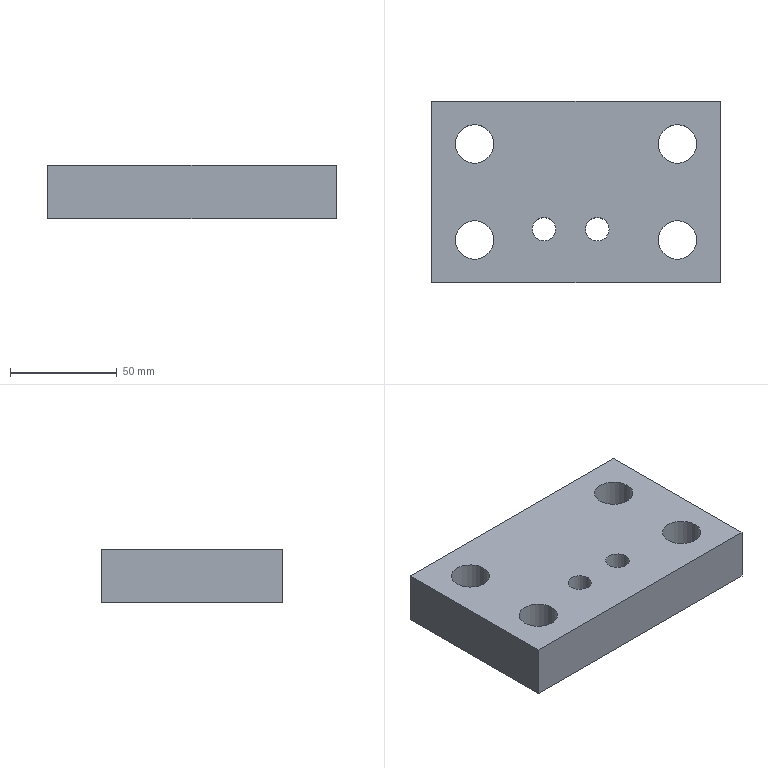Part | NX | features solid 2 | 1 solid | 16 faces | box 135 x 85 x 25 mm | volume 252850 mm3 | plane 8 | cylinder 8 | commonest cylinder face diameters 18 x6 11 x2
STEP:
#1=CARTESIAN_POINT('',(616.5,-425.,130.));
#2=VERTEX_POINT('',#1);
#3=CARTESIAN_POINT('',(607.5,-425.,130.));
#4=DIRECTION('',(0.,0.,-1.));
#5=DIRECTION('',(1.,0.,0.));
#6=AXIS2_PLACEMENT_3D('',#3,#4,#5);
#7=CIRCLE('',#6,9.);
#8=EDGE_CURVE('',#2,#2,#7,.T.);
#9=ORIENTED_EDGE('',*,*,#8,.F.);
#10=EDGE_LOOP('',(#9));
#11=FACE_BOUND('',#10,.T.);
#12=CARTESIAN_POINT('',(591.5,-425.,130.));
#13=VERTEX_POINT('',#12);
#14=CARTESIAN_POINT('',(582.5,-425.,130.));
#15=DIRECTION('',(0.,0.,-1.));
#16=DIRECTION('',(1.,0.,0.));
#17=AXIS2_PLACEMENT_3D('',#14,#15,#16);
#18=CIRCLE('',#17,9.);
#19=EDGE_CURVE('',#13,#13,#18,.T.);
#20=ORIENTED_EDGE('',*,*,#19,.F.);
#21=EDGE_LOOP('',(#20));
#22=FACE_BOUND('',#21,.T.);
#23=CARTESIAN_POINT('',(541.,-385.,130.));
#24=VERTEX_POINT('',#23);
#25=CARTESIAN_POINT('',(550.,-385.,130.));
#26=DIRECTION('',(0.,0.,-1.));
#27=DIRECTION('',(-1.,0.,0.));
#28=AXIS2_PLACEMENT_3D('',#25,#26,#27);
#29=CIRCLE('',#28,9.);
#30=EDGE_CURVE('',#24,#24,#29,.T.);
#31=ORIENTED_EDGE('',*,*,#30,.F.);
#32=EDGE_LOOP('',(#31));
#33=FACE_BOUND('',#32,.T.);
#34=CARTESIAN_POINT('',(541.,-430.,130.));
#35=VERTEX_POINT('',#34);
#36=CARTESIAN_POINT('',(550.,-430.,130.));
#37=DIRECTION('',(0.,0.,-1.));
#38=DIRECTION('',(-1.,0.,0.));
#39=AXIS2_PLACEMENT_3D('',#36,#37,#38);
#40=CIRCLE('',#39,9.);
#41=EDGE_CURVE('',#35,#35,#40,.T.);
#42=ORIENTED_EDGE('',*,*,#41,.F.);
#43=EDGE_LOOP('',(#42));
#44=FACE_BOUND('',#43,.T.);
#45=CARTESIAN_POINT('',(636.,-430.,130.));
#46=VERTEX_POINT('',#45);
#47=CARTESIAN_POINT('',(645.,-430.,130.));
#48=DIRECTION('',(0.,0.,-1.));
#49=DIRECTION('',(-1.,0.,0.));
#50=AXIS2_PLACEMENT_3D('',#47,#48,#49);
#51=CIRCLE('',#50,9.);
#52=EDGE_CURVE('',#46,#46,#51,.T.);
#53=ORIENTED_EDGE('',*,*,#52,.F.);
#54=EDGE_LOOP('',(#53));
#55=FACE_BOUND('',#54,.T.);
#56=CARTESIAN_POINT('',(636.,-385.,130.));
#57=VERTEX_POINT('',#56);
#58=CARTESIAN_POINT('',(645.,-385.,130.));
#59=DIRECTION('',(0.,0.,-1.));
#60=DIRECTION('',(-1.,0.,0.));
#61=AXIS2_PLACEMENT_3D('',#58,#59,#60);
#62=CIRCLE('',#61,9.);
#63=EDGE_CURVE('',#57,#57,#62,.T.);
#64=ORIENTED_EDGE('',*,*,#63,.F.);
#65=EDGE_LOOP('',(#64));
#66=FACE_BOUND('',#65,.T.);
#67=CARTESIAN_POINT('',(530.,-365.,130.));
#68=VERTEX_POINT('',#67);
#69=CARTESIAN_POINT('',(530.,-450.,130.));
#70=VERTEX_POINT('',#69);
#71=CARTESIAN_POINT('',(530.,-425.,130.));
#72=DIRECTION('',(0.,1.,0.));
#73=VECTOR('',#72,1000.);
#74=LINE('',#71,#73);
#75=EDGE_CURVE('',#68,#70,#74,.F.);
#76=ORIENTED_EDGE('',*,*,#75,.F.);
#77=CARTESIAN_POINT('',(665.,-365.,130.));
#78=VERTEX_POINT('',#77);
#79=CARTESIAN_POINT('',(555.,-365.,130.));
#80=DIRECTION('',(1.,0.,0.));
#81=VECTOR('',#80,1000.);
#82=LINE('',#79,#81);
#83=EDGE_CURVE('',#68,#78,#82,.T.);
#84=ORIENTED_EDGE('',*,*,#83,.T.);
#85=CARTESIAN_POINT('',(665.,-450.,130.));
#86=VERTEX_POINT('',#85);
#87=CARTESIAN_POINT('',(665.,-425.,130.));
#88=DIRECTION('',(0.,-1.,0.));
#89=VECTOR('',#88,1000.);
#90=LINE('',#87,#89);
#91=EDGE_CURVE('',#78,#86,#90,.T.);
#92=ORIENTED_EDGE('',*,*,#91,.T.);
#93=CARTESIAN_POINT('',(555.,-450.,130.));
#94=DIRECTION('',(1.,0.,0.));
#95=VECTOR('',#94,1000.);
#96=LINE('',#93,#95);
#97=EDGE_CURVE('',#70,#86,#96,.T.);
#98=ORIENTED_EDGE('',*,*,#97,.F.);
#99=EDGE_LOOP('',(#76,#84,#92,#98));
#100=FACE_BOUND('',#99,.T.);
#101=CARTESIAN_POINT('',(555.,-425.,130.));
#102=DIRECTION('',(0.,0.,-1.));
#103=DIRECTION('',(1.,0.,0.));
#104=AXIS2_PLACEMENT_3D('',#101,#102,#103);
#105=PLANE('',#104);
#106=ADVANCED_FACE('',(#11,#22,#33,#44,#55,#66,#100),#105,.T.);
#107=ORIENTED_EDGE('',*,*,#91,.F.);
#108=CARTESIAN_POINT('',(665.,-365.,155.));
#109=VERTEX_POINT('',#108);
#110=CARTESIAN_POINT('',(665.,-365.,130.));
#111=DIRECTION('',(0.,0.,1.));
#112=VECTOR('',#111,1000.);
#113=LINE('',#110,#112);
#114=EDGE_CURVE('',#78,#109,#113,.T.);
#115=ORIENTED_EDGE('',*,*,#114,.T.);
#116=CARTESIAN_POINT('',(665.,-450.,155.));
#117=VERTEX_POINT('',#116);
#118=CARTESIAN_POINT('',(665.,-425.,155.));
#119=DIRECTION('',(0.,1.,0.));
#120=VECTOR('',#119,1000.);
#121=LINE('',#118,#120);
#122=EDGE_CURVE('',#109,#117,#121,.F.);
#123=ORIENTED_EDGE('',*,*,#122,.T.);
#124=CARTESIAN_POINT('',(665.,-450.,130.));
#125=DIRECTION('',(0.,0.,1.));
#126=VECTOR('',#125,1000.);
#127=LINE('',#124,#126);
#128=EDGE_CURVE('',#86,#117,#127,.T.);
#129=ORIENTED_EDGE('',*,*,#128,.F.);
#130=EDGE_LOOP('',(#107,#115,#123,#129));
#131=FACE_BOUND('',#130,.T.);
#132=CARTESIAN_POINT('',(665.,-425.,130.));
#133=DIRECTION('',(1.,0.,0.));
#134=DIRECTION('',(0.,0.,1.));
#135=AXIS2_PLACEMENT_3D('',#132,#133,#134);
#136=PLANE('',#135);
#137=ADVANCED_FACE('',(#131),#136,.T.);
#138=CARTESIAN_POINT('',(602.,-425.,155.));
#139=VERTEX_POINT('',#138);
#140=CARTESIAN_POINT('',(607.5,-425.,155.));
#141=DIRECTION('',(0.,0.,1.));
#142=DIRECTION('',(-1.,0.,0.));
#143=AXIS2_PLACEMENT_3D('',#140,#141,#142);
#144=CIRCLE('',#143,5.5);
#145=EDGE_CURVE('',#139,#139,#144,.F.);
#146=ORIENTED_EDGE('',*,*,#145,.T.);
#147=EDGE_LOOP('',(#146));
#148=FACE_BOUND('',#147,.T.);
#149=CARTESIAN_POINT('',(577.,-425.,155.));
#150=VERTEX_POINT('',#149);
#151=CARTESIAN_POINT('',(582.5,-425.,155.));
#152=DIRECTION('',(0.,0.,1.));
#153=DIRECTION('',(-1.,0.,0.));
#154=AXIS2_PLACEMENT_3D('',#151,#152,#153);
#155=CIRCLE('',#154,5.5);
#156=EDGE_CURVE('',#150,#150,#155,.F.);
#157=ORIENTED_EDGE('',*,*,#156,.T.);
#158=EDGE_LOOP('',(#157));
#159=FACE_BOUND('',#158,.T.);
#160=CARTESIAN_POINT('',(541.,-385.,155.));
#161=VERTEX_POINT('',#160);
#162=CARTESIAN_POINT('',(550.,-385.,155.));
#163=DIRECTION('',(0.,0.,-1.));
#164=DIRECTION('',(-1.,0.,0.));
#165=AXIS2_PLACEMENT_3D('',#162,#163,#164);
#166=CIRCLE('',#165,9.);
#167=EDGE_CURVE('',#161,#161,#166,.T.);
#168=ORIENTED_EDGE('',*,*,#167,.T.);
#169=EDGE_LOOP('',(#168));
#170=FACE_BOUND('',#169,.T.);
#171=CARTESIAN_POINT('',(541.,-430.,155.));
#172=VERTEX_POINT('',#171);
#173=CARTESIAN_POINT('',(550.,-430.,155.));
#174=DIRECTION('',(0.,0.,-1.));
#175=DIRECTION('',(-1.,0.,0.));
#176=AXIS2_PLACEMENT_3D('',#173,#174,#175);
#177=CIRCLE('',#176,9.);
#178=EDGE_CURVE('',#172,#172,#177,.T.);
#179=ORIENTED_EDGE('',*,*,#178,.T.);
#180=EDGE_LOOP('',(#179));
#181=FACE_BOUND('',#180,.T.);
#182=CARTESIAN_POINT('',(636.,-430.,155.));
#183=VERTEX_POINT('',#182);
#184=CARTESIAN_POINT('',(645.,-430.,155.));
#185=DIRECTION('',(0.,0.,-1.));
#186=DIRECTION('',(-1.,0.,0.));
#187=AXIS2_PLACEMENT_3D('',#184,#185,#186);
#188=CIRCLE('',#187,9.);
#189=EDGE_CURVE('',#183,#183,#188,.T.);
#190=ORIENTED_EDGE('',*,*,#189,.T.);
#191=EDGE_LOOP('',(#190));
#192=FACE_BOUND('',#191,.T.);
#193=CARTESIAN_POINT('',(636.,-385.,155.));
#194=VERTEX_POINT('',#193);
#195=CARTESIAN_POINT('',(645.,-385.,155.));
#196=DIRECTION('',(0.,0.,-1.));
#197=DIRECTION('',(-1.,0.,0.));
#198=AXIS2_PLACEMENT_3D('',#195,#196,#197);
#199=CIRCLE('',#198,9.);
#200=EDGE_CURVE('',#194,#194,#199,.T.);
#201=ORIENTED_EDGE('',*,*,#200,.T.);
#202=EDGE_LOOP('',(#201));
#203=FACE_BOUND('',#202,.T.);
#204=ORIENTED_EDGE('',*,*,#122,.F.);
#205=CARTESIAN_POINT('',(530.,-365.,155.));
#206=VERTEX_POINT('',#205);
#207=CARTESIAN_POINT('',(555.,-365.,155.));
#208=DIRECTION('',(-1.,0.,0.));
#209=VECTOR('',#208,1000.);
#210=LINE('',#207,#209);
#211=EDGE_CURVE('',#206,#109,#210,.F.);
#212=ORIENTED_EDGE('',*,*,#211,.F.);
#213=CARTESIAN_POINT('',(530.,-450.,155.));
#214=VERTEX_POINT('',#213);
#215=CARTESIAN_POINT('',(530.,-425.,155.));
#216=DIRECTION('',(0.,-1.,0.));
#217=VECTOR('',#216,1000.);
#218=LINE('',#215,#217);
#219=EDGE_CURVE('',#206,#214,#218,.T.);
#220=ORIENTED_EDGE('',*,*,#219,.T.);
#221=CARTESIAN_POINT('',(555.,-450.,155.));
#222=DIRECTION('',(-1.,0.,0.));
#223=VECTOR('',#222,1000.);
#224=LINE('',#221,#223);
#225=EDGE_CURVE('',#214,#117,#224,.F.);
#226=ORIENTED_EDGE('',*,*,#225,.T.);
#227=EDGE_LOOP('',(#204,#212,#220,#226));
#228=FACE_BOUND('',#227,.T.);
#229=CARTESIAN_POINT('',(555.,-425.,155.));
#230=DIRECTION('',(0.,0.,-1.));
#231=DIRECTION('',(1.,0.,0.));
#232=AXIS2_PLACEMENT_3D('',#229,#230,#231);
#233=PLANE('',#232);
#234=ADVANCED_FACE('',(#148,#159,#170,#181,#192,#203,#228),#233,.F.);
#235=CARTESIAN_POINT('',(530.,-365.,130.));
#236=DIRECTION('',(0.,0.,-1.));
#237=VECTOR('',#236,1000.);
#238=LINE('',#235,#237);
#239=EDGE_CURVE('',#68,#206,#238,.F.);
#240=ORIENTED_EDGE('',*,*,#239,.F.);
#241=ORIENTED_EDGE('',*,*,#75,.T.);
#242=CARTESIAN_POINT('',(530.,-450.,130.));
#243=DIRECTION('',(0.,0.,-1.));
#244=VECTOR('',#243,1000.);
#245=LINE('',#242,#244);
#246=EDGE_CURVE('',#70,#214,#245,.F.);
#247=ORIENTED_EDGE('',*,*,#246,.T.);
#248=ORIENTED_EDGE('',*,*,#219,.F.);
#249=EDGE_LOOP('',(#240,#241,#247,#248));
#250=FACE_BOUND('',#249,.T.);
#251=CARTESIAN_POINT('',(530.,-425.,130.));
#252=DIRECTION('',(1.,0.,0.));
#253=DIRECTION('',(0.,0.,1.));
#254=AXIS2_PLACEMENT_3D('',#251,#252,#253);
#255=PLANE('',#254);
#256=ADVANCED_FACE('',(#250),#255,.F.);
#257=ORIENTED_EDGE('',*,*,#225,.F.);
#258=ORIENTED_EDGE('',*,*,#246,.F.);
#259=ORIENTED_EDGE('',*,*,#97,.T.);
#260=ORIENTED_EDGE('',*,*,#128,.T.);
#261=EDGE_LOOP('',(#257,#258,#259,#260));
#262=FACE_BOUND('',#261,.T.);
#263=CARTESIAN_POINT('',(555.,-450.,130.));
#264=DIRECTION('',(0.,-1.,0.));
#265=DIRECTION('',(0.,0.,-1.));
#266=AXIS2_PLACEMENT_3D('',#263,#264,#265);
#267=PLANE('',#266);
#268=ADVANCED_FACE('',(#262),#267,.T.);
#269=ORIENTED_EDGE('',*,*,#211,.T.);
#270=ORIENTED_EDGE('',*,*,#114,.F.);
#271=ORIENTED_EDGE('',*,*,#83,.F.);
#272=ORIENTED_EDGE('',*,*,#239,.T.);
#273=EDGE_LOOP('',(#269,#270,#271,#272));
#274=FACE_BOUND('',#273,.T.);
#275=CARTESIAN_POINT('',(555.,-365.,130.));
#276=DIRECTION('',(0.,-1.,0.));
#277=DIRECTION('',(0.,0.,-1.));
#278=AXIS2_PLACEMENT_3D('',#275,#276,#277);
#279=PLANE('',#278);
#280=ADVANCED_FACE('',(#274),#279,.F.);
#281=ORIENTED_EDGE('',*,*,#63,.T.);
#282=EDGE_LOOP('',(#281));
#283=FACE_BOUND('',#282,.T.);
#284=ORIENTED_EDGE('',*,*,#200,.F.);
#285=EDGE_LOOP('',(#284));
#286=FACE_BOUND('',#285,.T.);
#287=CARTESIAN_POINT('',(645.,-385.,155.));
#288=DIRECTION('',(0.,0.,-1.));
#289=DIRECTION('',(-1.,0.,0.));
#290=AXIS2_PLACEMENT_3D('',#287,#288,#289);
#291=CYLINDRICAL_SURFACE('',#290,9.);
#292=ADVANCED_FACE('',(#283,#286),#291,.F.);
#293=ORIENTED_EDGE('',*,*,#52,.T.);
#294=EDGE_LOOP('',(#293));
#295=FACE_BOUND('',#294,.T.);
#296=ORIENTED_EDGE('',*,*,#189,.F.);
#297=EDGE_LOOP('',(#296));
#298=FACE_BOUND('',#297,.T.);
#299=CARTESIAN_POINT('',(645.,-430.,155.));
#300=DIRECTION('',(0.,0.,-1.));
#301=DIRECTION('',(-1.,0.,0.));
#302=AXIS2_PLACEMENT_3D('',#299,#300,#301);
#303=CYLINDRICAL_SURFACE('',#302,9.);
#304=ADVANCED_FACE('',(#295,#298),#303,.F.);
#305=ORIENTED_EDGE('',*,*,#41,.T.);
#306=EDGE_LOOP('',(#305));
#307=FACE_BOUND('',#306,.T.);
#308=ORIENTED_EDGE('',*,*,#178,.F.);
#309=EDGE_LOOP('',(#308));
#310=FACE_BOUND('',#309,.T.);
#311=CARTESIAN_POINT('',(550.,-430.,155.));
#312=DIRECTION('',(0.,0.,-1.));
#313=DIRECTION('',(-1.,0.,0.));
#314=AXIS2_PLACEMENT_3D('',#311,#312,#313);
#315=CYLINDRICAL_SURFACE('',#314,9.);
#316=ADVANCED_FACE('',(#307,#310),#315,.F.);
#317=ORIENTED_EDGE('',*,*,#30,.T.);
#318=EDGE_LOOP('',(#317));
#319=FACE_BOUND('',#318,.T.);
#320=ORIENTED_EDGE('',*,*,#167,.F.);
#321=EDGE_LOOP('',(#320));
#322=FACE_BOUND('',#321,.T.);
#323=CARTESIAN_POINT('',(550.,-385.,155.));
#324=DIRECTION('',(0.,0.,-1.));
#325=DIRECTION('',(-1.,0.,0.));
#326=AXIS2_PLACEMENT_3D('',#323,#324,#325);
#327=CYLINDRICAL_SURFACE('',#326,9.);
#328=ADVANCED_FACE('',(#319,#322),#327,.F.);
#329=ORIENTED_EDGE('',*,*,#156,.F.);
#330=EDGE_LOOP('',(#329));
#331=FACE_BOUND('',#330,.T.);
#332=CARTESIAN_POINT('',(588.,-425.,142.));
#333=VERTEX_POINT('',#332);
#334=CARTESIAN_POINT('',(582.5,-425.,142.));
#335=DIRECTION('',(0.,0.,-1.));
#336=DIRECTION('',(1.,0.,0.));
#337=AXIS2_PLACEMENT_3D('',#334,#335,#336);
#338=CIRCLE('',#337,5.5);
#339=EDGE_CURVE('',#333,#333,#338,.T.);
#340=ORIENTED_EDGE('',*,*,#339,.T.);
#341=EDGE_LOOP('',(#340));
#342=FACE_BOUND('',#341,.T.);
#343=CARTESIAN_POINT('',(582.5,-425.,180.));
#344=DIRECTION('',(0.,0.,1.));
#345=DIRECTION('',(1.,0.,0.));
#346=AXIS2_PLACEMENT_3D('',#343,#344,#345);
#347=CYLINDRICAL_SURFACE('',#346,5.5);
#348=ADVANCED_FACE('',(#331,#342),#347,.F.);
#349=ORIENTED_EDGE('',*,*,#339,.F.);
#350=EDGE_LOOP('',(#349));
#351=FACE_BOUND('',#350,.T.);
#352=CARTESIAN_POINT('',(591.5,-425.,142.));
#353=VERTEX_POINT('',#352);
#354=CARTESIAN_POINT('',(582.5,-425.,142.));
#355=DIRECTION('',(0.,0.,-1.));
#356=DIRECTION('',(1.,0.,0.));
#357=AXIS2_PLACEMENT_3D('',#354,#355,#356);
#358=CIRCLE('',#357,9.);
#359=EDGE_CURVE('',#353,#353,#358,.T.);
#360=ORIENTED_EDGE('',*,*,#359,.T.);
#361=EDGE_LOOP('',(#360));
#362=FACE_BOUND('',#361,.T.);
#363=CARTESIAN_POINT('',(582.5,-425.,142.));
#364=DIRECTION('',(0.,0.,1.));
#365=DIRECTION('',(1.,0.,0.));
#366=AXIS2_PLACEMENT_3D('',#363,#364,#365);
#367=PLANE('',#366);
#368=ADVANCED_FACE('',(#351,#362),#367,.F.);
#369=ORIENTED_EDGE('',*,*,#359,.F.);
#370=EDGE_LOOP('',(#369));
#371=FACE_BOUND('',#370,.T.);
#372=ORIENTED_EDGE('',*,*,#19,.T.);
#373=EDGE_LOOP('',(#372));
#374=FACE_BOUND('',#373,.T.);
#375=CARTESIAN_POINT('',(582.5,-425.,130.));
#376=DIRECTION('',(0.,0.,1.));
#377=DIRECTION('',(1.,0.,0.));
#378=AXIS2_PLACEMENT_3D('',#375,#376,#377);
#379=CYLINDRICAL_SURFACE('',#378,9.);
#380=ADVANCED_FACE('',(#371,#374),#379,.F.);
#381=ORIENTED_EDGE('',*,*,#145,.F.);
#382=EDGE_LOOP('',(#381));
#383=FACE_BOUND('',#382,.T.);
#384=CARTESIAN_POINT('',(613.,-425.,142.));
#385=VERTEX_POINT('',#384);
#386=CARTESIAN_POINT('',(607.5,-425.,142.));
#387=DIRECTION('',(0.,0.,-1.));
#388=DIRECTION('',(1.,0.,0.));
#389=AXIS2_PLACEMENT_3D('',#386,#387,#388);
#390=CIRCLE('',#389,5.5);
#391=EDGE_CURVE('',#385,#385,#390,.T.);
#392=ORIENTED_EDGE('',*,*,#391,.T.);
#393=EDGE_LOOP('',(#392));
#394=FACE_BOUND('',#393,.T.);
#395=CARTESIAN_POINT('',(607.5,-425.,180.));
#396=DIRECTION('',(0.,0.,1.));
#397=DIRECTION('',(1.,0.,0.));
#398=AXIS2_PLACEMENT_3D('',#395,#396,#397);
#399=CYLINDRICAL_SURFACE('',#398,5.5);
#400=ADVANCED_FACE('',(#383,#394),#399,.F.);
#401=ORIENTED_EDGE('',*,*,#391,.F.);
#402=EDGE_LOOP('',(#401));
#403=FACE_BOUND('',#402,.T.);
#404=CARTESIAN_POINT('',(616.5,-425.,142.));
#405=VERTEX_POINT('',#404);
#406=CARTESIAN_POINT('',(607.5,-425.,142.));
#407=DIRECTION('',(0.,0.,-1.));
#408=DIRECTION('',(1.,0.,0.));
#409=AXIS2_PLACEMENT_3D('',#406,#407,#408);
#410=CIRCLE('',#409,9.);
#411=EDGE_CURVE('',#405,#405,#410,.T.);
#412=ORIENTED_EDGE('',*,*,#411,.T.);
#413=EDGE_LOOP('',(#412));
#414=FACE_BOUND('',#413,.T.);
#415=CARTESIAN_POINT('',(607.5,-425.,142.));
#416=DIRECTION('',(0.,0.,1.));
#417=DIRECTION('',(1.,0.,0.));
#418=AXIS2_PLACEMENT_3D('',#415,#416,#417);
#419=PLANE('',#418);
#420=ADVANCED_FACE('',(#403,#414),#419,.F.);
#421=ORIENTED_EDGE('',*,*,#411,.F.);
#422=EDGE_LOOP('',(#421));
#423=FACE_BOUND('',#422,.T.);
#424=ORIENTED_EDGE('',*,*,#8,.T.);
#425=EDGE_LOOP('',(#424));
#426=FACE_BOUND('',#425,.T.);
#427=CARTESIAN_POINT('',(607.5,-425.,130.));
#428=DIRECTION('',(0.,0.,1.));
#429=DIRECTION('',(1.,0.,0.));
#430=AXIS2_PLACEMENT_3D('',#427,#428,#429);
#431=CYLINDRICAL_SURFACE('',#430,9.);
#432=ADVANCED_FACE('',(#423,#426),#431,.F.);
#433=CLOSED_SHELL('',(#106,#137,#234,#256,#268,#280,#292,#304,#316,#328,#348,#368,#380,#400,#420,#432));
#434=MANIFOLD_SOLID_BREP('',#433);
#435=(LENGTH_UNIT()NAMED_UNIT(*)SI_UNIT(.MILLI.,.METRE.));
#436=UNCERTAINTY_MEASURE_WITH_UNIT(LENGTH_MEASURE(0.00001),#435,'','');
#437=(NAMED_UNIT(*)PLANE_ANGLE_UNIT()SI_UNIT($,.RADIAN.));
#438=(NAMED_UNIT(*)SI_UNIT($,.STERADIAN.)SOLID_ANGLE_UNIT());
#439=(GEOMETRIC_REPRESENTATION_CONTEXT(3)GLOBAL_UNCERTAINTY_ASSIGNED_CONTEXT((#436))GLOBAL_UNIT_ASSIGNED_CONTEXT((#435,#437,#438))REPRESENTATION_CONTEXT('',''));
#440=ADVANCED_BREP_SHAPE_REPRESENTATION('',(#434),#439);